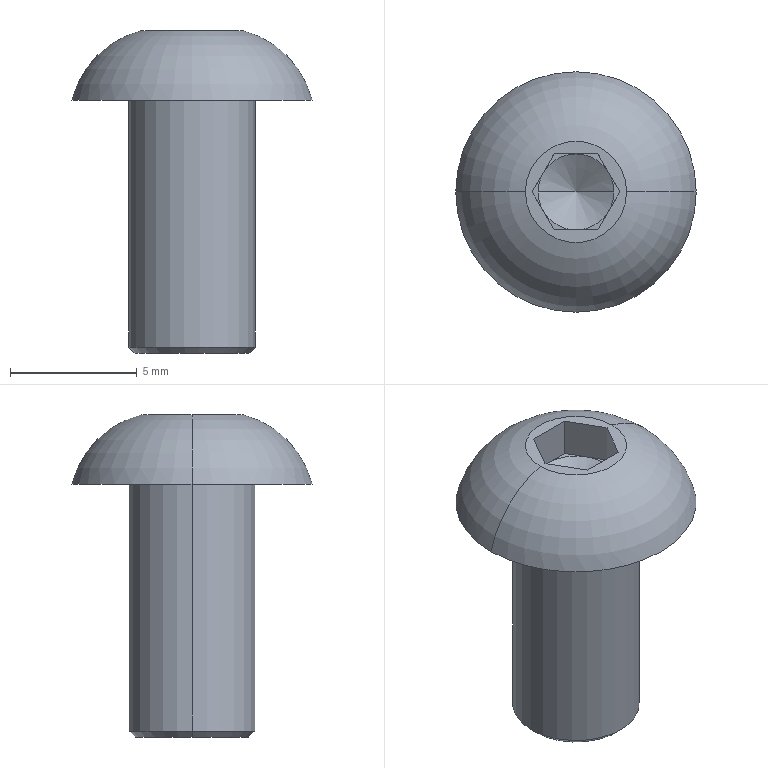Part | NX | features BREP 1 | 1 solid | 23 faces | box 9.5 x 9.5 x 12.75 mm | volume 316.744 mm3 | plane 15 | cone 4 | torus 2 | cylinder 2 | commonest cylinder face diameters 5 x2
STEP:
#1=CARTESIAN_POINT('',(0.,0.,0.324));
#2=VERTEX_POINT('',#1);
#3=CARTESIAN_POINT('',(-1.5,0.,1.19));
#4=VERTEX_POINT('',#3);
#5=CARTESIAN_POINT('',(-1.5,0.,1.19));
#6=DIRECTION('',(-0.866,0.,0.5));
#7=VECTOR('',#6,1000.);
#8=LINE('',#5,#7);
#9=EDGE_CURVE('',#2,#4,#8,.T.);
#10=ORIENTED_EDGE('',*,*,#9,.F.);
#11=CARTESIAN_POINT('',(1.5,0.,1.19));
#12=VERTEX_POINT('',#11);
#13=CARTESIAN_POINT('',(1.5,0.,1.19));
#14=DIRECTION('',(0.866,0.,0.5));
#15=VECTOR('',#14,1000.);
#16=LINE('',#13,#15);
#17=EDGE_CURVE('',#2,#12,#16,.T.);
#18=ORIENTED_EDGE('',*,*,#17,.T.);
#19=CARTESIAN_POINT('',(1.299,0.75,1.19));
#20=VERTEX_POINT('',#19);
#21=CARTESIAN_POINT('',(0.,0.,1.19));
#22=DIRECTION('',(0.,0.,1.));
#23=DIRECTION('',(1.,0.,0.));
#24=AXIS2_PLACEMENT_3D('',#21,#22,#23);
#25=CIRCLE('',#24,1.5);
#26=EDGE_CURVE('',#12,#20,#25,.T.);
#27=ORIENTED_EDGE('',*,*,#26,.T.);
#28=CARTESIAN_POINT('',(0.,1.5,1.19));
#29=VERTEX_POINT('',#28);
#30=CARTESIAN_POINT('',(0.,0.,1.19));
#31=DIRECTION('',(0.,0.,1.));
#32=DIRECTION('',(1.,0.,0.));
#33=AXIS2_PLACEMENT_3D('',#30,#31,#32);
#34=CIRCLE('',#33,1.5);
#35=EDGE_CURVE('',#20,#29,#34,.T.);
#36=ORIENTED_EDGE('',*,*,#35,.T.);
#37=CARTESIAN_POINT('',(-1.299,0.75,1.19));
#38=VERTEX_POINT('',#37);
#39=CARTESIAN_POINT('',(0.,0.,1.19));
#40=DIRECTION('',(0.,0.,-1.));
#41=DIRECTION('',(-1.,0.,0.));
#42=AXIS2_PLACEMENT_3D('',#39,#40,#41);
#43=CIRCLE('',#42,1.5);
#44=EDGE_CURVE('',#38,#29,#43,.T.);
#45=ORIENTED_EDGE('',*,*,#44,.F.);
#46=CARTESIAN_POINT('',(0.,0.,1.19));
#47=DIRECTION('',(0.,0.,1.));
#48=DIRECTION('',(1.,0.,0.));
#49=AXIS2_PLACEMENT_3D('',#46,#47,#48);
#50=CIRCLE('',#49,1.5);
#51=EDGE_CURVE('',#38,#4,#50,.T.);
#52=ORIENTED_EDGE('',*,*,#51,.T.);
#53=EDGE_LOOP('',(#10,#18,#27,#36,#45,#52));
#54=FACE_BOUND('',#53,.T.);
#55=CARTESIAN_POINT('',(0.,0.,1.19));
#56=DIRECTION('',(0.,0.,1.));
#57=DIRECTION('',(-1.,0.,0.));
#58=AXIS2_PLACEMENT_3D('',#55,#56,#57);
#59=CONICAL_SURFACE('',#58,1.5,1.047);
#60=ADVANCED_FACE('',(#54),#59,.F.);
#61=CARTESIAN_POINT('',(-2.25,0.,-10.));
#62=VERTEX_POINT('',#61);
#63=CARTESIAN_POINT('',(2.25,0.,-10.));
#64=VERTEX_POINT('',#63);
#65=CARTESIAN_POINT('',(0.,0.,-10.));
#66=DIRECTION('',(0.,0.,1.));
#67=DIRECTION('',(-1.,0.,0.));
#68=AXIS2_PLACEMENT_3D('',#65,#66,#67);
#69=CIRCLE('',#68,2.25);
#70=EDGE_CURVE('',#62,#64,#69,.T.);
#71=ORIENTED_EDGE('',*,*,#70,.T.);
#72=CARTESIAN_POINT('',(2.5,0.,-9.75));
#73=VERTEX_POINT('',#72);
#74=CARTESIAN_POINT('',(2.5,0.,-9.75));
#75=DIRECTION('',(0.7071,0.,0.7071));
#76=VECTOR('',#75,1000.);
#77=LINE('',#74,#76);
#78=EDGE_CURVE('',#64,#73,#77,.T.);
#79=ORIENTED_EDGE('',*,*,#78,.T.);
#80=CARTESIAN_POINT('',(-2.5,0.,-9.75));
#81=VERTEX_POINT('',#80);
#82=CARTESIAN_POINT('',(0.,0.,-9.75));
#83=DIRECTION('',(0.,0.,-1.));
#84=DIRECTION('',(-1.,0.,0.));
#85=AXIS2_PLACEMENT_3D('',#82,#83,#84);
#86=CIRCLE('',#85,2.5);
#87=EDGE_CURVE('',#73,#81,#86,.T.);
#88=ORIENTED_EDGE('',*,*,#87,.T.);
#89=CARTESIAN_POINT('',(-2.5,0.,-9.75));
#90=DIRECTION('',(-0.7071,0.,0.7071));
#91=VECTOR('',#90,1000.);
#92=LINE('',#89,#91);
#93=EDGE_CURVE('',#62,#81,#92,.T.);
#94=ORIENTED_EDGE('',*,*,#93,.F.);
#95=EDGE_LOOP('',(#71,#79,#88,#94));
#96=FACE_BOUND('',#95,.T.);
#97=CARTESIAN_POINT('',(0.,0.,-9.75));
#98=DIRECTION('',(0.,0.,1.));
#99=DIRECTION('',(-1.,0.,0.));
#100=AXIS2_PLACEMENT_3D('',#97,#98,#99);
#101=CONICAL_SURFACE('',#100,2.5,0.7854);
#102=ADVANCED_FACE('',(#96),#101,.T.);
#103=CARTESIAN_POINT('',(4.75,0.,0.));
#104=VERTEX_POINT('',#103);
#105=CARTESIAN_POINT('',(-4.75,0.,0.));
#106=VERTEX_POINT('',#105);
#107=CARTESIAN_POINT('',(0.,0.,0.));
#108=DIRECTION('',(0.,0.,-1.));
#109=DIRECTION('',(-1.,0.,0.));
#110=AXIS2_PLACEMENT_3D('',#107,#108,#109);
#111=CIRCLE('',#110,4.75);
#112=EDGE_CURVE('',#104,#106,#111,.T.);
#113=ORIENTED_EDGE('',*,*,#112,.F.);
#114=CARTESIAN_POINT('',(2.,0.,2.75));
#115=VERTEX_POINT('',#114);
#116=CARTESIAN_POINT('',(1.066,0.,-0.9335));
#117=DIRECTION('',(0.,-1.,0.));
#118=DIRECTION('',(1.,0.,0.));
#119=AXIS2_PLACEMENT_3D('',#116,#117,#118);
#120=CIRCLE('',#119,3.8);
#121=EDGE_CURVE('',#104,#115,#120,.T.);
#122=ORIENTED_EDGE('',*,*,#121,.T.);
#123=CARTESIAN_POINT('',(-2.,0.,2.75));
#124=VERTEX_POINT('',#123);
#125=CARTESIAN_POINT('',(0.,0.,2.75));
#126=DIRECTION('',(0.,0.,-1.));
#127=DIRECTION('',(-1.,0.,0.));
#128=AXIS2_PLACEMENT_3D('',#125,#126,#127);
#129=CIRCLE('',#128,2.);
#130=EDGE_CURVE('',#115,#124,#129,.T.);
#131=ORIENTED_EDGE('',*,*,#130,.T.);
#132=CARTESIAN_POINT('',(-1.066,0.,-0.9335));
#133=DIRECTION('',(0.,1.,0.));
#134=DIRECTION('',(0.,0.,1.));
#135=AXIS2_PLACEMENT_3D('',#132,#133,#134);
#136=CIRCLE('',#135,3.8);
#137=EDGE_CURVE('',#106,#124,#136,.T.);
#138=ORIENTED_EDGE('',*,*,#137,.F.);
#139=EDGE_LOOP('',(#113,#122,#131,#138));
#140=FACE_BOUND('',#139,.T.);
#141=CARTESIAN_POINT('',(0.,0.,-0.9335));
#142=DIRECTION('',(0.,0.,1.));
#143=DIRECTION('',(-1.,0.,0.));
#144=AXIS2_PLACEMENT_3D('',#141,#142,#143);
#145=DEGENERATE_TOROIDAL_SURFACE('',#144,1.066,3.8,.T.);
#146=ADVANCED_FACE('',(#140),#145,.T.);
#147=ORIENTED_EDGE('',*,*,#87,.F.);
#148=CARTESIAN_POINT('',(2.5,0.,0.));
#149=VERTEX_POINT('',#148);
#150=CARTESIAN_POINT('',(2.5,0.,-10.));
#151=DIRECTION('',(0.,0.,1.));
#152=VECTOR('',#151,1000.);
#153=LINE('',#150,#152);
#154=EDGE_CURVE('',#73,#149,#153,.T.);
#155=ORIENTED_EDGE('',*,*,#154,.T.);
#156=CARTESIAN_POINT('',(-2.5,0.,0.));
#157=VERTEX_POINT('',#156);
#158=CARTESIAN_POINT('',(0.,0.,0.));
#159=DIRECTION('',(0.,0.,1.));
#160=DIRECTION('',(1.,0.,0.));
#161=AXIS2_PLACEMENT_3D('',#158,#159,#160);
#162=CIRCLE('',#161,2.5);
#163=EDGE_CURVE('',#157,#149,#162,.T.);
#164=ORIENTED_EDGE('',*,*,#163,.F.);
#165=CARTESIAN_POINT('',(-2.5,0.,-10.));
#166=DIRECTION('',(0.,0.,1.));
#167=VECTOR('',#166,1000.);
#168=LINE('',#165,#167);
#169=EDGE_CURVE('',#81,#157,#168,.T.);
#170=ORIENTED_EDGE('',*,*,#169,.F.);
#171=EDGE_LOOP('',(#147,#155,#164,#170));
#172=FACE_BOUND('',#171,.T.);
#173=CARTESIAN_POINT('',(0.,0.,-10.));
#174=DIRECTION('',(0.,0.,1.));
#175=DIRECTION('',(-1.,0.,0.));
#176=AXIS2_PLACEMENT_3D('',#173,#174,#175);
#177=CYLINDRICAL_SURFACE('',#176,2.5);
#178=ADVANCED_FACE('',(#172),#177,.T.);
#179=CARTESIAN_POINT('',(0.866,1.5,1.19));
#180=VERTEX_POINT('',#179);
#181=CARTESIAN_POINT('',(1.732,0.,1.19));
#182=DIRECTION('',(-0.5,0.866,0.));
#183=VECTOR('',#182,1000.);
#184=LINE('',#181,#183);
#185=EDGE_CURVE('',#20,#180,#184,.T.);
#186=ORIENTED_EDGE('',*,*,#185,.T.);
#187=CARTESIAN_POINT('',(0.866,1.5,1.19));
#188=DIRECTION('',(-1.,0.,0.));
#189=VECTOR('',#188,1000.);
#190=LINE('',#187,#189);
#191=EDGE_CURVE('',#180,#29,#190,.T.);
#192=ORIENTED_EDGE('',*,*,#191,.T.);
#193=ORIENTED_EDGE('',*,*,#35,.F.);
#194=EDGE_LOOP('',(#186,#192,#193));
#195=FACE_BOUND('',#194,.T.);
#196=CARTESIAN_POINT('',(0.,0.,1.19));
#197=DIRECTION('',(0.,0.,-1.));
#198=DIRECTION('',(0.,-1.,0.));
#199=AXIS2_PLACEMENT_3D('',#196,#197,#198);
#200=PLANE('',#199);
#201=ADVANCED_FACE('',(#195),#200,.F.);
#202=CARTESIAN_POINT('',(-0.866,1.5,1.19));
#203=VERTEX_POINT('',#202);
#204=CARTESIAN_POINT('',(0.866,1.5,1.19));
#205=DIRECTION('',(-1.,0.,0.));
#206=VECTOR('',#205,1000.);
#207=LINE('',#204,#206);
#208=EDGE_CURVE('',#29,#203,#207,.T.);
#209=ORIENTED_EDGE('',*,*,#208,.T.);
#210=CARTESIAN_POINT('',(-0.866,1.5,1.19));
#211=DIRECTION('',(-0.5,-0.866,0.));
#212=VECTOR('',#211,1000.);
#213=LINE('',#210,#212);
#214=EDGE_CURVE('',#203,#38,#213,.T.);
#215=ORIENTED_EDGE('',*,*,#214,.T.);
#216=ORIENTED_EDGE('',*,*,#44,.T.);
#217=EDGE_LOOP('',(#209,#215,#216));
#218=FACE_BOUND('',#217,.T.);
#219=CARTESIAN_POINT('',(0.,0.,1.19));
#220=DIRECTION('',(0.,0.,-1.));
#221=DIRECTION('',(0.,-1.,0.));
#222=AXIS2_PLACEMENT_3D('',#219,#220,#221);
#223=PLANE('',#222);
#224=ADVANCED_FACE('',(#218),#223,.F.);
#225=CARTESIAN_POINT('',(-1.732,0.,1.19));
#226=VERTEX_POINT('',#225);
#227=CARTESIAN_POINT('',(-0.866,1.5,1.19));
#228=DIRECTION('',(-0.5,-0.866,0.));
#229=VECTOR('',#228,1000.);
#230=LINE('',#227,#229);
#231=EDGE_CURVE('',#38,#226,#230,.T.);
#232=ORIENTED_EDGE('',*,*,#231,.T.);
#233=CARTESIAN_POINT('',(-1.299,-0.75,1.19));
#234=VERTEX_POINT('',#233);
#235=CARTESIAN_POINT('',(-1.732,0.,1.19));
#236=DIRECTION('',(0.5,-0.866,0.));
#237=VECTOR('',#236,1000.);
#238=LINE('',#235,#237);
#239=EDGE_CURVE('',#226,#234,#238,.T.);
#240=ORIENTED_EDGE('',*,*,#239,.T.);
#241=CARTESIAN_POINT('',(0.,0.,1.19));
#242=DIRECTION('',(0.,0.,1.));
#243=DIRECTION('',(1.,0.,0.));
#244=AXIS2_PLACEMENT_3D('',#241,#242,#243);
#245=CIRCLE('',#244,1.5);
#246=EDGE_CURVE('',#4,#234,#245,.T.);
#247=ORIENTED_EDGE('',*,*,#246,.F.);
#248=ORIENTED_EDGE('',*,*,#51,.F.);
#249=EDGE_LOOP('',(#232,#240,#247,#248));
#250=FACE_BOUND('',#249,.T.);
#251=CARTESIAN_POINT('',(0.,0.,1.19));
#252=DIRECTION('',(0.,0.,-1.));
#253=DIRECTION('',(0.,-1.,0.));
#254=AXIS2_PLACEMENT_3D('',#251,#252,#253);
#255=PLANE('',#254);
#256=ADVANCED_FACE('',(#250),#255,.F.);
#257=CARTESIAN_POINT('',(-0.866,-1.5,1.19));
#258=VERTEX_POINT('',#257);
#259=CARTESIAN_POINT('',(-1.732,0.,1.19));
#260=DIRECTION('',(0.5,-0.866,0.));
#261=VECTOR('',#260,1000.);
#262=LINE('',#259,#261);
#263=EDGE_CURVE('',#234,#258,#262,.T.);
#264=ORIENTED_EDGE('',*,*,#263,.T.);
#265=CARTESIAN_POINT('',(0.,-1.5,1.19));
#266=VERTEX_POINT('',#265);
#267=CARTESIAN_POINT('',(-0.866,-1.5,1.19));
#268=DIRECTION('',(1.,0.,0.));
#269=VECTOR('',#268,1000.);
#270=LINE('',#267,#269);
#271=EDGE_CURVE('',#258,#266,#270,.T.);
#272=ORIENTED_EDGE('',*,*,#271,.T.);
#273=CARTESIAN_POINT('',(0.,0.,1.19));
#274=DIRECTION('',(0.,0.,1.));
#275=DIRECTION('',(1.,0.,0.));
#276=AXIS2_PLACEMENT_3D('',#273,#274,#275);
#277=CIRCLE('',#276,1.5);
#278=EDGE_CURVE('',#234,#266,#277,.T.);
#279=ORIENTED_EDGE('',*,*,#278,.F.);
#280=EDGE_LOOP('',(#264,#272,#279));
#281=FACE_BOUND('',#280,.T.);
#282=CARTESIAN_POINT('',(0.,0.,1.19));
#283=DIRECTION('',(0.,0.,-1.));
#284=DIRECTION('',(0.,-1.,0.));
#285=AXIS2_PLACEMENT_3D('',#282,#283,#284);
#286=PLANE('',#285);
#287=ADVANCED_FACE('',(#281),#286,.F.);
#288=CARTESIAN_POINT('',(0.866,-1.5,1.19));
#289=VERTEX_POINT('',#288);
#290=CARTESIAN_POINT('',(-0.866,-1.5,1.19));
#291=DIRECTION('',(1.,0.,0.));
#292=VECTOR('',#291,1000.);
#293=LINE('',#290,#292);
#294=EDGE_CURVE('',#266,#289,#293,.T.);
#295=ORIENTED_EDGE('',*,*,#294,.T.);
#296=CARTESIAN_POINT('',(1.299,-0.75,1.19));
#297=VERTEX_POINT('',#296);
#298=CARTESIAN_POINT('',(0.866,-1.5,1.19));
#299=DIRECTION('',(0.5,0.866,0.));
#300=VECTOR('',#299,1000.);
#301=LINE('',#298,#300);
#302=EDGE_CURVE('',#289,#297,#301,.T.);
#303=ORIENTED_EDGE('',*,*,#302,.T.);
#304=CARTESIAN_POINT('',(0.,0.,1.19));
#305=DIRECTION('',(0.,0.,1.));
#306=DIRECTION('',(1.,0.,0.));
#307=AXIS2_PLACEMENT_3D('',#304,#305,#306);
#308=CIRCLE('',#307,1.5);
#309=EDGE_CURVE('',#266,#297,#308,.T.);
#310=ORIENTED_EDGE('',*,*,#309,.F.);
#311=EDGE_LOOP('',(#295,#303,#310));
#312=FACE_BOUND('',#311,.T.);
#313=CARTESIAN_POINT('',(0.,0.,1.19));
#314=DIRECTION('',(0.,0.,-1.));
#315=DIRECTION('',(0.,-1.,0.));
#316=AXIS2_PLACEMENT_3D('',#313,#314,#315);
#317=PLANE('',#316);
#318=ADVANCED_FACE('',(#312),#317,.F.);
#319=CARTESIAN_POINT('',(0.,0.,2.75));
#320=DIRECTION('',(0.,0.,-1.));
#321=DIRECTION('',(-1.,0.,0.));
#322=AXIS2_PLACEMENT_3D('',#319,#320,#321);
#323=CIRCLE('',#322,2.);
#324=EDGE_CURVE('',#124,#115,#323,.T.);
#325=ORIENTED_EDGE('',*,*,#324,.F.);
#326=ORIENTED_EDGE('',*,*,#130,.F.);
#327=EDGE_LOOP('',(#325,#326));
#328=FACE_BOUND('',#327,.T.);
#329=CARTESIAN_POINT('',(1.732,0.,2.75));
#330=VERTEX_POINT('',#329);
#331=CARTESIAN_POINT('',(0.866,1.5,2.75));
#332=VERTEX_POINT('',#331);
#333=CARTESIAN_POINT('',(1.732,0.,2.75));
#334=DIRECTION('',(-0.5,0.866,0.));
#335=VECTOR('',#334,1000.);
#336=LINE('',#333,#335);
#337=EDGE_CURVE('',#330,#332,#336,.T.);
#338=ORIENTED_EDGE('',*,*,#337,.F.);
#339=CARTESIAN_POINT('',(0.866,-1.5,2.75));
#340=VERTEX_POINT('',#339);
#341=CARTESIAN_POINT('',(0.866,-1.5,2.75));
#342=DIRECTION('',(0.5,0.866,0.));
#343=VECTOR('',#342,1000.);
#344=LINE('',#341,#343);
#345=EDGE_CURVE('',#340,#330,#344,.T.);
#346=ORIENTED_EDGE('',*,*,#345,.F.);
#347=CARTESIAN_POINT('',(-0.866,-1.5,2.75));
#348=VERTEX_POINT('',#347);
#349=CARTESIAN_POINT('',(-0.866,-1.5,2.75));
#350=DIRECTION('',(1.,0.,0.));
#351=VECTOR('',#350,1000.);
#352=LINE('',#349,#351);
#353=EDGE_CURVE('',#348,#340,#352,.T.);
#354=ORIENTED_EDGE('',*,*,#353,.F.);
#355=CARTESIAN_POINT('',(-1.732,0.,2.75));
#356=VERTEX_POINT('',#355);
#357=CARTESIAN_POINT('',(-1.732,0.,2.75));
#358=DIRECTION('',(0.5,-0.866,0.));
#359=VECTOR('',#358,1000.);
#360=LINE('',#357,#359);
#361=EDGE_CURVE('',#356,#348,#360,.T.);
#362=ORIENTED_EDGE('',*,*,#361,.F.);
#363=CARTESIAN_POINT('',(-0.866,1.5,2.75));
#364=VERTEX_POINT('',#363);
#365=CARTESIAN_POINT('',(-0.866,1.5,2.75));
#366=DIRECTION('',(-0.5,-0.866,0.));
#367=VECTOR('',#366,1000.);
#368=LINE('',#365,#367);
#369=EDGE_CURVE('',#364,#356,#368,.T.);
#370=ORIENTED_EDGE('',*,*,#369,.F.);
#371=CARTESIAN_POINT('',(0.866,1.5,2.75));
#372=DIRECTION('',(-1.,0.,0.));
#373=VECTOR('',#372,1000.);
#374=LINE('',#371,#373);
#375=EDGE_CURVE('',#332,#364,#374,.T.);
#376=ORIENTED_EDGE('',*,*,#375,.F.);
#377=EDGE_LOOP('',(#338,#346,#354,#362,#370,#376));
#378=FACE_BOUND('',#377,.T.);
#379=CARTESIAN_POINT('',(0.,0.,2.75));
#380=DIRECTION('',(0.,0.,-1.));
#381=DIRECTION('',(0.,-1.,0.));
#382=AXIS2_PLACEMENT_3D('',#379,#380,#381);
#383=PLANE('',#382);
#384=ADVANCED_FACE('',(#328,#378),#383,.F.);
#385=CARTESIAN_POINT('',(0.,0.,0.));
#386=DIRECTION('',(0.,0.,-1.));
#387=DIRECTION('',(-1.,0.,0.));
#388=AXIS2_PLACEMENT_3D('',#385,#386,#387);
#389=CIRCLE('',#388,4.75);
#390=EDGE_CURVE('',#106,#104,#389,.T.);
#391=ORIENTED_EDGE('',*,*,#390,.T.);
#392=ORIENTED_EDGE('',*,*,#112,.T.);
#393=EDGE_LOOP('',(#391,#392));
#394=FACE_BOUND('',#393,.T.);
#395=ORIENTED_EDGE('',*,*,#163,.T.);
#396=CARTESIAN_POINT('',(0.,0.,0.));
#397=DIRECTION('',(0.,0.,1.));
#398=DIRECTION('',(1.,0.,0.));
#399=AXIS2_PLACEMENT_3D('',#396,#397,#398);
#400=CIRCLE('',#399,2.5);
#401=EDGE_CURVE('',#149,#157,#400,.T.);
#402=ORIENTED_EDGE('',*,*,#401,.T.);
#403=EDGE_LOOP('',(#395,#402));
#404=FACE_BOUND('',#403,.T.);
#405=CARTESIAN_POINT('',(0.,0.,0.));
#406=DIRECTION('',(0.,0.,-1.));
#407=DIRECTION('',(0.,-1.,0.));
#408=AXIS2_PLACEMENT_3D('',#405,#406,#407);
#409=PLANE('',#408);
#410=ADVANCED_FACE('',(#394,#404),#409,.T.);
#411=ORIENTED_EDGE('',*,*,#154,.F.);
#412=CARTESIAN_POINT('',(0.,0.,-9.75));
#413=DIRECTION('',(0.,0.,-1.));
#414=DIRECTION('',(-1.,0.,0.));
#415=AXIS2_PLACEMENT_3D('',#412,#413,#414);
#416=CIRCLE('',#415,2.5);
#417=EDGE_CURVE('',#81,#73,#416,.T.);
#418=ORIENTED_EDGE('',*,*,#417,.F.);
#419=ORIENTED_EDGE('',*,*,#169,.T.);
#420=ORIENTED_EDGE('',*,*,#401,.F.);
#421=EDGE_LOOP('',(#411,#418,#419,#420));
#422=FACE_BOUND('',#421,.T.);
#423=CARTESIAN_POINT('',(0.,0.,-10.));
#424=DIRECTION('',(0.,0.,1.));
#425=DIRECTION('',(-1.,0.,0.));
#426=AXIS2_PLACEMENT_3D('',#423,#424,#425);
#427=CYLINDRICAL_SURFACE('',#426,2.5);
#428=ADVANCED_FACE('',(#422),#427,.T.);
#429=ORIENTED_EDGE('',*,*,#70,.F.);
#430=CARTESIAN_POINT('',(0.,0.,-10.));
#431=DIRECTION('',(0.,0.,1.));
#432=DIRECTION('',(-1.,0.,0.));
#433=AXIS2_PLACEMENT_3D('',#430,#431,#432);
#434=CIRCLE('',#433,2.25);
#435=EDGE_CURVE('',#64,#62,#434,.T.);
#436=ORIENTED_EDGE('',*,*,#435,.F.);
#437=EDGE_LOOP('',(#429,#436));
#438=FACE_BOUND('',#437,.T.);
#439=CARTESIAN_POINT('',(0.,0.,-10.));
#440=DIRECTION('',(0.,0.,1.));
#441=DIRECTION('',(1.,0.,0.));
#442=AXIS2_PLACEMENT_3D('',#439,#440,#441);
#443=PLANE('',#442);
#444=ADVANCED_FACE('',(#438),#443,.F.);
#445=ORIENTED_EDGE('',*,*,#121,.F.);
#446=ORIENTED_EDGE('',*,*,#390,.F.);
#447=ORIENTED_EDGE('',*,*,#137,.T.);
#448=ORIENTED_EDGE('',*,*,#324,.T.);
#449=EDGE_LOOP('',(#445,#446,#447,#448));
#450=FACE_BOUND('',#449,.T.);
#451=CARTESIAN_POINT('',(0.,0.,-0.9335));
#452=DIRECTION('',(0.,0.,1.));
#453=DIRECTION('',(-1.,0.,0.));
#454=AXIS2_PLACEMENT_3D('',#451,#452,#453);
#455=DEGENERATE_TOROIDAL_SURFACE('',#454,1.066,3.8,.T.);
#456=ADVANCED_FACE('',(#450),#455,.T.);
#457=ORIENTED_EDGE('',*,*,#78,.F.);
#458=ORIENTED_EDGE('',*,*,#435,.T.);
#459=ORIENTED_EDGE('',*,*,#93,.T.);
#460=ORIENTED_EDGE('',*,*,#417,.T.);
#461=EDGE_LOOP('',(#457,#458,#459,#460));
#462=FACE_BOUND('',#461,.T.);
#463=CARTESIAN_POINT('',(0.,0.,-9.75));
#464=DIRECTION('',(0.,0.,1.));
#465=DIRECTION('',(-1.,0.,0.));
#466=AXIS2_PLACEMENT_3D('',#463,#464,#465);
#467=CONICAL_SURFACE('',#466,2.5,0.7854);
#468=ADVANCED_FACE('',(#462),#467,.T.);
#469=ORIENTED_EDGE('',*,*,#337,.T.);
#470=CARTESIAN_POINT('',(0.866,1.5,1.19));
#471=DIRECTION('',(0.,0.,1.));
#472=VECTOR('',#471,1000.);
#473=LINE('',#470,#472);
#474=EDGE_CURVE('',#180,#332,#473,.T.);
#475=ORIENTED_EDGE('',*,*,#474,.F.);
#476=ORIENTED_EDGE('',*,*,#185,.F.);
#477=CARTESIAN_POINT('',(1.732,0.,1.19));
#478=VERTEX_POINT('',#477);
#479=CARTESIAN_POINT('',(1.732,0.,1.19));
#480=DIRECTION('',(-0.5,0.866,0.));
#481=VECTOR('',#480,1000.);
#482=LINE('',#479,#481);
#483=EDGE_CURVE('',#478,#20,#482,.T.);
#484=ORIENTED_EDGE('',*,*,#483,.F.);
#485=CARTESIAN_POINT('',(1.732,0.,1.19));
#486=DIRECTION('',(0.,0.,1.));
#487=VECTOR('',#486,1000.);
#488=LINE('',#485,#487);
#489=EDGE_CURVE('',#478,#330,#488,.T.);
#490=ORIENTED_EDGE('',*,*,#489,.T.);
#491=EDGE_LOOP('',(#469,#475,#476,#484,#490));
#492=FACE_BOUND('',#491,.T.);
#493=CARTESIAN_POINT('',(1.732,0.,1.19));
#494=DIRECTION('',(-0.866,-0.5,0.));
#495=DIRECTION('',(-0.5,0.866,0.));
#496=AXIS2_PLACEMENT_3D('',#493,#494,#495);
#497=PLANE('',#496);
#498=ADVANCED_FACE('',(#492),#497,.T.);
#499=ORIENTED_EDGE('',*,*,#375,.T.);
#500=CARTESIAN_POINT('',(-0.866,1.5,1.19));
#501=DIRECTION('',(0.,0.,1.));
#502=VECTOR('',#501,1000.);
#503=LINE('',#500,#502);
#504=EDGE_CURVE('',#203,#364,#503,.T.);
#505=ORIENTED_EDGE('',*,*,#504,.F.);
#506=ORIENTED_EDGE('',*,*,#208,.F.);
#507=ORIENTED_EDGE('',*,*,#191,.F.);
#508=ORIENTED_EDGE('',*,*,#474,.T.);
#509=EDGE_LOOP('',(#499,#505,#506,#507,#508));
#510=FACE_BOUND('',#509,.T.);
#511=CARTESIAN_POINT('',(0.866,1.5,1.19));
#512=DIRECTION('',(0.,-1.,0.));
#513=DIRECTION('',(0.,0.,-1.));
#514=AXIS2_PLACEMENT_3D('',#511,#512,#513);
#515=PLANE('',#514);
#516=ADVANCED_FACE('',(#510),#515,.T.);
#517=ORIENTED_EDGE('',*,*,#369,.T.);
#518=CARTESIAN_POINT('',(-1.732,0.,1.19));
#519=DIRECTION('',(0.,0.,1.));
#520=VECTOR('',#519,1000.);
#521=LINE('',#518,#520);
#522=EDGE_CURVE('',#226,#356,#521,.T.);
#523=ORIENTED_EDGE('',*,*,#522,.F.);
#524=ORIENTED_EDGE('',*,*,#231,.F.);
#525=ORIENTED_EDGE('',*,*,#214,.F.);
#526=ORIENTED_EDGE('',*,*,#504,.T.);
#527=EDGE_LOOP('',(#517,#523,#524,#525,#526));
#528=FACE_BOUND('',#527,.T.);
#529=CARTESIAN_POINT('',(-0.866,1.5,1.19));
#530=DIRECTION('',(0.866,-0.5,0.));
#531=DIRECTION('',(0.,0.,-1.));
#532=AXIS2_PLACEMENT_3D('',#529,#530,#531);
#533=PLANE('',#532);
#534=ADVANCED_FACE('',(#528),#533,.T.);
#535=ORIENTED_EDGE('',*,*,#361,.T.);
#536=CARTESIAN_POINT('',(-0.866,-1.5,1.19));
#537=DIRECTION('',(0.,0.,1.));
#538=VECTOR('',#537,1000.);
#539=LINE('',#536,#538);
#540=EDGE_CURVE('',#258,#348,#539,.T.);
#541=ORIENTED_EDGE('',*,*,#540,.F.);
#542=ORIENTED_EDGE('',*,*,#263,.F.);
#543=ORIENTED_EDGE('',*,*,#239,.F.);
#544=ORIENTED_EDGE('',*,*,#522,.T.);
#545=EDGE_LOOP('',(#535,#541,#542,#543,#544));
#546=FACE_BOUND('',#545,.T.);
#547=CARTESIAN_POINT('',(-1.732,0.,1.19));
#548=DIRECTION('',(0.866,0.5,0.));
#549=DIRECTION('',(0.,0.,-1.));
#550=AXIS2_PLACEMENT_3D('',#547,#548,#549);
#551=PLANE('',#550);
#552=ADVANCED_FACE('',(#546),#551,.T.);
#553=ORIENTED_EDGE('',*,*,#353,.T.);
#554=CARTESIAN_POINT('',(0.866,-1.5,1.19));
#555=DIRECTION('',(0.,0.,1.));
#556=VECTOR('',#555,1000.);
#557=LINE('',#554,#556);
#558=EDGE_CURVE('',#289,#340,#557,.T.);
#559=ORIENTED_EDGE('',*,*,#558,.F.);
#560=ORIENTED_EDGE('',*,*,#294,.F.);
#561=ORIENTED_EDGE('',*,*,#271,.F.);
#562=ORIENTED_EDGE('',*,*,#540,.T.);
#563=EDGE_LOOP('',(#553,#559,#560,#561,#562));
#564=FACE_BOUND('',#563,.T.);
#565=CARTESIAN_POINT('',(-0.866,-1.5,1.19));
#566=DIRECTION('',(0.,1.,0.));
#567=DIRECTION('',(1.,0.,0.));
#568=AXIS2_PLACEMENT_3D('',#565,#566,#567);
#569=PLANE('',#568);
#570=ADVANCED_FACE('',(#564),#569,.T.);
#571=ORIENTED_EDGE('',*,*,#345,.T.);
#572=ORIENTED_EDGE('',*,*,#489,.F.);
#573=CARTESIAN_POINT('',(0.866,-1.5,1.19));
#574=DIRECTION('',(0.5,0.866,0.));
#575=VECTOR('',#574,1000.);
#576=LINE('',#573,#575);
#577=EDGE_CURVE('',#297,#478,#576,.T.);
#578=ORIENTED_EDGE('',*,*,#577,.F.);
#579=ORIENTED_EDGE('',*,*,#302,.F.);
#580=ORIENTED_EDGE('',*,*,#558,.T.);
#581=EDGE_LOOP('',(#571,#572,#578,#579,#580));
#582=FACE_BOUND('',#581,.T.);
#583=CARTESIAN_POINT('',(0.866,-1.5,1.19));
#584=DIRECTION('',(-0.866,0.5,0.));
#585=DIRECTION('',(0.,0.,1.));
#586=AXIS2_PLACEMENT_3D('',#583,#584,#585);
#587=PLANE('',#586);
#588=ADVANCED_FACE('',(#582),#587,.T.);
#589=ORIENTED_EDGE('',*,*,#577,.T.);
#590=ORIENTED_EDGE('',*,*,#483,.T.);
#591=ORIENTED_EDGE('',*,*,#26,.F.);
#592=CARTESIAN_POINT('',(0.,0.,1.19));
#593=DIRECTION('',(0.,0.,1.));
#594=DIRECTION('',(1.,0.,0.));
#595=AXIS2_PLACEMENT_3D('',#592,#593,#594);
#596=CIRCLE('',#595,1.5);
#597=EDGE_CURVE('',#297,#12,#596,.T.);
#598=ORIENTED_EDGE('',*,*,#597,.F.);
#599=EDGE_LOOP('',(#589,#590,#591,#598));
#600=FACE_BOUND('',#599,.T.);
#601=CARTESIAN_POINT('',(0.,0.,1.19));
#602=DIRECTION('',(0.,0.,-1.));
#603=DIRECTION('',(0.,-1.,0.));
#604=AXIS2_PLACEMENT_3D('',#601,#602,#603);
#605=PLANE('',#604);
#606=ADVANCED_FACE('',(#600),#605,.F.);
#607=ORIENTED_EDGE('',*,*,#17,.F.);
#608=ORIENTED_EDGE('',*,*,#9,.T.);
#609=ORIENTED_EDGE('',*,*,#246,.T.);
#610=ORIENTED_EDGE('',*,*,#278,.T.);
#611=ORIENTED_EDGE('',*,*,#309,.T.);
#612=ORIENTED_EDGE('',*,*,#597,.T.);
#613=EDGE_LOOP('',(#607,#608,#609,#610,#611,#612));
#614=FACE_BOUND('',#613,.T.);
#615=CARTESIAN_POINT('',(0.,0.,1.19));
#616=DIRECTION('',(0.,0.,1.));
#617=DIRECTION('',(-1.,0.,0.));
#618=AXIS2_PLACEMENT_3D('',#615,#616,#617);
#619=CONICAL_SURFACE('',#618,1.5,1.047);
#620=ADVANCED_FACE('',(#614),#619,.F.);
#621=CLOSED_SHELL('',(#60,#102,#146,#178,#201,#224,#256,#287,#318,#384,#410,#428,#444,#456,#468,#498,#516,#534,#552,#570,#588,#606,#620));
#622=MANIFOLD_SOLID_BREP('',#621);
#623=(LENGTH_UNIT()NAMED_UNIT(*)SI_UNIT(.MILLI.,.METRE.));
#624=UNCERTAINTY_MEASURE_WITH_UNIT(LENGTH_MEASURE(0.00001),#623,'','');
#625=(NAMED_UNIT(*)PLANE_ANGLE_UNIT()SI_UNIT($,.RADIAN.));
#626=(NAMED_UNIT(*)SI_UNIT($,.STERADIAN.)SOLID_ANGLE_UNIT());
#627=(GEOMETRIC_REPRESENTATION_CONTEXT(3)GLOBAL_UNCERTAINTY_ASSIGNED_CONTEXT((#624))GLOBAL_UNIT_ASSIGNED_CONTEXT((#623,#625,#626))REPRESENTATION_CONTEXT('',''));
#628=ADVANCED_BREP_SHAPE_REPRESENTATION('',(#622),#627);